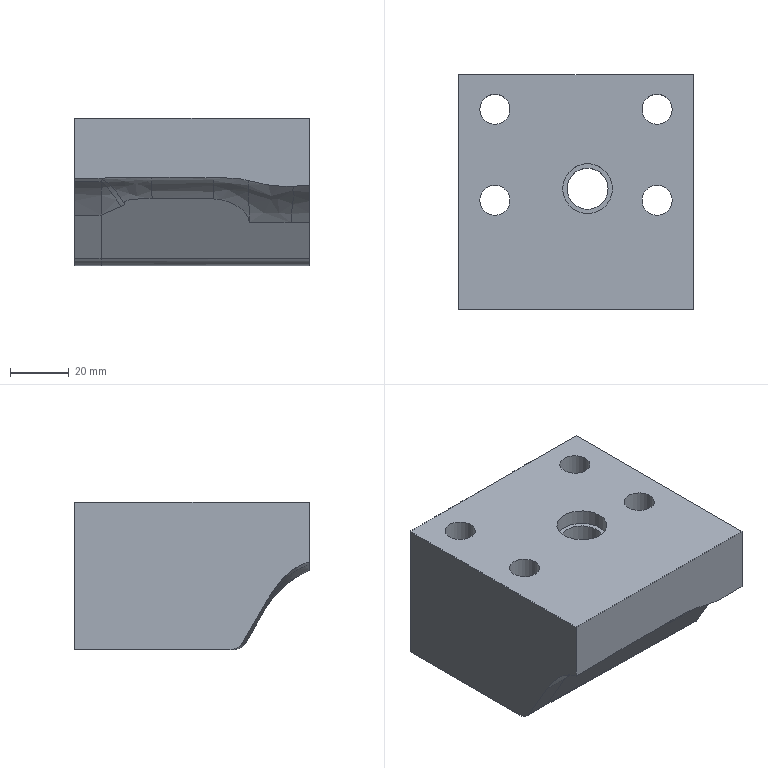Part | NX | features solid 2 | 1 solid | 35 faces | box 80 x 80.002 x 50.25 mm | volume 250607 mm3 | plane 13 | cylinder 12 | spline 10 | commonest cylinder face diameters 17 x5 10.3 x4 10 x1 14 x1 30 x1